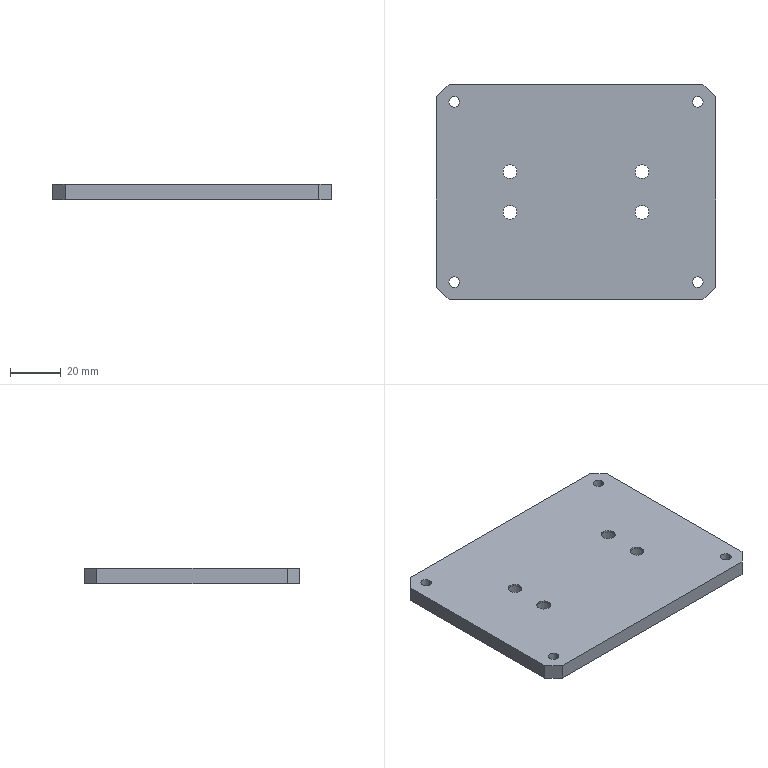Part | SolidWorks | features HoleWzd 2, Chamfer 1, Extrusion 1 | 1 solid | 38 faces | box 110 x 85 x 6 mm | volume 53736 mm3 | cylinder 24 | plane 14 | commonest cylinder face diameters 4.2 x8 5.5 x8 10 x8
STEP:
#1=CARTESIAN_POINT('',(-71.134,24.385,0.));
#2=VERTEX_POINT('',#1);
#3=CARTESIAN_POINT('',(-66.934,24.385,0.));
#4=VERTEX_POINT('',#3);
#5=CARTESIAN_POINT('',(-69.034,24.385,0.));
#6=DIRECTION('',(0.,0.,1.));
#7=DIRECTION('',(1.,0.,0.));
#8=AXIS2_PLACEMENT_3D('',#5,#6,#7);
#9=CIRCLE('',#8,2.1);
#10=EDGE_CURVE('',#2,#4,#9,.T.);
#11=ORIENTED_EDGE('',*,*,#10,.F.);
#12=CARTESIAN_POINT('',(-71.134,24.385,6.));
#13=VERTEX_POINT('',#12);
#14=CARTESIAN_POINT('',(-71.134,24.385,6.));
#15=DIRECTION('',(0.,0.,1.));
#16=VECTOR('',#15,1000.);
#17=LINE('',#14,#16);
#18=EDGE_CURVE('',#2,#13,#17,.T.);
#19=ORIENTED_EDGE('',*,*,#18,.T.);
#20=CARTESIAN_POINT('',(-66.934,24.385,6.));
#21=VERTEX_POINT('',#20);
#22=CARTESIAN_POINT('',(-69.034,24.385,6.));
#23=DIRECTION('',(0.,0.,1.));
#24=DIRECTION('',(1.,0.,0.));
#25=AXIS2_PLACEMENT_3D('',#22,#23,#24);
#26=CIRCLE('',#25,2.1);
#27=EDGE_CURVE('',#13,#21,#26,.T.);
#28=ORIENTED_EDGE('',*,*,#27,.T.);
#29=CARTESIAN_POINT('',(-66.934,24.385,6.));
#30=DIRECTION('',(0.,0.,1.));
#31=VECTOR('',#30,1000.);
#32=LINE('',#29,#31);
#33=EDGE_CURVE('',#4,#21,#32,.T.);
#34=ORIENTED_EDGE('',*,*,#33,.F.);
#35=EDGE_LOOP('',(#11,#19,#28,#34));
#36=FACE_OUTER_BOUND('',#35,.T.);
#37=CARTESIAN_POINT('',(-69.034,24.385,6.));
#38=DIRECTION('',(0.,0.,1.));
#39=DIRECTION('',(1.,0.,0.));
#40=AXIS2_PLACEMENT_3D('',#37,#38,#39);
#41=CYLINDRICAL_SURFACE('',#40,2.1);
#42=ADVANCED_FACE('',(#36),#41,.F.);
#43=CARTESIAN_POINT('',(24.866,24.385,0.));
#44=VERTEX_POINT('',#43);
#45=CARTESIAN_POINT('',(29.066,24.385,0.));
#46=VERTEX_POINT('',#45);
#47=CARTESIAN_POINT('',(26.966,24.385,0.));
#48=DIRECTION('',(0.,0.,1.));
#49=DIRECTION('',(1.,0.,0.));
#50=AXIS2_PLACEMENT_3D('',#47,#48,#49);
#51=CIRCLE('',#50,2.1);
#52=EDGE_CURVE('',#44,#46,#51,.T.);
#53=ORIENTED_EDGE('',*,*,#52,.F.);
#54=CARTESIAN_POINT('',(24.866,24.385,6.));
#55=VERTEX_POINT('',#54);
#56=CARTESIAN_POINT('',(24.866,24.385,6.));
#57=DIRECTION('',(0.,0.,1.));
#58=VECTOR('',#57,1000.);
#59=LINE('',#56,#58);
#60=EDGE_CURVE('',#44,#55,#59,.T.);
#61=ORIENTED_EDGE('',*,*,#60,.T.);
#62=CARTESIAN_POINT('',(29.066,24.385,6.));
#63=VERTEX_POINT('',#62);
#64=CARTESIAN_POINT('',(26.966,24.385,6.));
#65=DIRECTION('',(0.,0.,1.));
#66=DIRECTION('',(1.,0.,0.));
#67=AXIS2_PLACEMENT_3D('',#64,#65,#66);
#68=CIRCLE('',#67,2.1);
#69=EDGE_CURVE('',#55,#63,#68,.T.);
#70=ORIENTED_EDGE('',*,*,#69,.T.);
#71=CARTESIAN_POINT('',(29.066,24.385,6.));
#72=DIRECTION('',(0.,0.,1.));
#73=VECTOR('',#72,1000.);
#74=LINE('',#71,#73);
#75=EDGE_CURVE('',#46,#63,#74,.T.);
#76=ORIENTED_EDGE('',*,*,#75,.F.);
#77=EDGE_LOOP('',(#53,#61,#70,#76));
#78=FACE_OUTER_BOUND('',#77,.T.);
#79=CARTESIAN_POINT('',(26.966,24.385,6.));
#80=DIRECTION('',(0.,0.,1.));
#81=DIRECTION('',(1.,0.,0.));
#82=AXIS2_PLACEMENT_3D('',#79,#80,#81);
#83=CYLINDRICAL_SURFACE('',#82,2.1);
#84=ADVANCED_FACE('',(#78),#83,.F.);
#85=CARTESIAN_POINT('',(24.866,-46.615,0.));
#86=VERTEX_POINT('',#85);
#87=CARTESIAN_POINT('',(29.066,-46.615,0.));
#88=VERTEX_POINT('',#87);
#89=CARTESIAN_POINT('',(26.966,-46.615,0.));
#90=DIRECTION('',(0.,0.,1.));
#91=DIRECTION('',(1.,0.,0.));
#92=AXIS2_PLACEMENT_3D('',#89,#90,#91);
#93=CIRCLE('',#92,2.1);
#94=EDGE_CURVE('',#86,#88,#93,.T.);
#95=ORIENTED_EDGE('',*,*,#94,.F.);
#96=CARTESIAN_POINT('',(24.866,-46.615,6.));
#97=VERTEX_POINT('',#96);
#98=CARTESIAN_POINT('',(24.866,-46.615,6.));
#99=DIRECTION('',(0.,0.,1.));
#100=VECTOR('',#99,1000.);
#101=LINE('',#98,#100);
#102=EDGE_CURVE('',#86,#97,#101,.T.);
#103=ORIENTED_EDGE('',*,*,#102,.T.);
#104=CARTESIAN_POINT('',(29.066,-46.615,6.));
#105=VERTEX_POINT('',#104);
#106=CARTESIAN_POINT('',(26.966,-46.615,6.));
#107=DIRECTION('',(0.,0.,1.));
#108=DIRECTION('',(1.,0.,0.));
#109=AXIS2_PLACEMENT_3D('',#106,#107,#108);
#110=CIRCLE('',#109,2.1);
#111=EDGE_CURVE('',#97,#105,#110,.T.);
#112=ORIENTED_EDGE('',*,*,#111,.T.);
#113=CARTESIAN_POINT('',(29.066,-46.615,6.));
#114=DIRECTION('',(0.,0.,1.));
#115=VECTOR('',#114,1000.);
#116=LINE('',#113,#115);
#117=EDGE_CURVE('',#88,#105,#116,.T.);
#118=ORIENTED_EDGE('',*,*,#117,.F.);
#119=EDGE_LOOP('',(#95,#103,#112,#118));
#120=FACE_OUTER_BOUND('',#119,.T.);
#121=CARTESIAN_POINT('',(26.966,-46.615,6.));
#122=DIRECTION('',(0.,0.,1.));
#123=DIRECTION('',(1.,0.,0.));
#124=AXIS2_PLACEMENT_3D('',#121,#122,#123);
#125=CYLINDRICAL_SURFACE('',#124,2.1);
#126=ADVANCED_FACE('',(#120),#125,.F.);
#127=CARTESIAN_POINT('',(-71.134,-46.615,0.));
#128=VERTEX_POINT('',#127);
#129=CARTESIAN_POINT('',(-66.934,-46.615,0.));
#130=VERTEX_POINT('',#129);
#131=CARTESIAN_POINT('',(-69.034,-46.615,0.));
#132=DIRECTION('',(0.,0.,1.));
#133=DIRECTION('',(1.,0.,0.));
#134=AXIS2_PLACEMENT_3D('',#131,#132,#133);
#135=CIRCLE('',#134,2.1);
#136=EDGE_CURVE('',#128,#130,#135,.T.);
#137=ORIENTED_EDGE('',*,*,#136,.F.);
#138=CARTESIAN_POINT('',(-71.134,-46.615,6.));
#139=VERTEX_POINT('',#138);
#140=CARTESIAN_POINT('',(-71.134,-46.615,6.));
#141=DIRECTION('',(0.,0.,1.));
#142=VECTOR('',#141,1000.);
#143=LINE('',#140,#142);
#144=EDGE_CURVE('',#128,#139,#143,.T.);
#145=ORIENTED_EDGE('',*,*,#144,.T.);
#146=CARTESIAN_POINT('',(-66.934,-46.615,6.));
#147=VERTEX_POINT('',#146);
#148=CARTESIAN_POINT('',(-69.034,-46.615,6.));
#149=DIRECTION('',(0.,0.,1.));
#150=DIRECTION('',(1.,0.,0.));
#151=AXIS2_PLACEMENT_3D('',#148,#149,#150);
#152=CIRCLE('',#151,2.1);
#153=EDGE_CURVE('',#139,#147,#152,.T.);
#154=ORIENTED_EDGE('',*,*,#153,.T.);
#155=CARTESIAN_POINT('',(-66.934,-46.615,6.));
#156=DIRECTION('',(0.,0.,1.));
#157=VECTOR('',#156,1000.);
#158=LINE('',#155,#157);
#159=EDGE_CURVE('',#130,#147,#158,.T.);
#160=ORIENTED_EDGE('',*,*,#159,.F.);
#161=EDGE_LOOP('',(#137,#145,#154,#160));
#162=FACE_OUTER_BOUND('',#161,.T.);
#163=CARTESIAN_POINT('',(-69.034,-46.615,6.));
#164=DIRECTION('',(0.,0.,1.));
#165=DIRECTION('',(1.,0.,0.));
#166=AXIS2_PLACEMENT_3D('',#163,#164,#165);
#167=CYLINDRICAL_SURFACE('',#166,2.1);
#168=ADVANCED_FACE('',(#162),#167,.F.);
#169=CARTESIAN_POINT('',(-42.034,-19.115,5.3));
#170=VERTEX_POINT('',#169);
#171=CARTESIAN_POINT('',(-52.034,-19.115,5.3));
#172=VERTEX_POINT('',#171);
#173=CARTESIAN_POINT('',(-47.034,-19.115,5.3));
#174=DIRECTION('',(0.,0.,-1.));
#175=DIRECTION('',(-1.,0.,0.));
#176=AXIS2_PLACEMENT_3D('',#173,#174,#175);
#177=CIRCLE('',#176,5.);
#178=EDGE_CURVE('',#170,#172,#177,.T.);
#179=ORIENTED_EDGE('',*,*,#178,.F.);
#180=CARTESIAN_POINT('',(-42.034,-19.115,0.));
#181=VERTEX_POINT('',#180);
#182=CARTESIAN_POINT('',(-42.034,-19.115,0.));
#183=DIRECTION('',(0.,0.,-1.));
#184=VECTOR('',#183,1000.);
#185=LINE('',#182,#184);
#186=EDGE_CURVE('',#170,#181,#185,.T.);
#187=ORIENTED_EDGE('',*,*,#186,.T.);
#188=CARTESIAN_POINT('',(-52.034,-19.115,0.));
#189=VERTEX_POINT('',#188);
#190=CARTESIAN_POINT('',(-47.034,-19.115,0.));
#191=DIRECTION('',(0.,0.,-1.));
#192=DIRECTION('',(-1.,0.,0.));
#193=AXIS2_PLACEMENT_3D('',#190,#191,#192);
#194=CIRCLE('',#193,5.);
#195=EDGE_CURVE('',#181,#189,#194,.T.);
#196=ORIENTED_EDGE('',*,*,#195,.T.);
#197=CARTESIAN_POINT('',(-52.034,-19.115,0.));
#198=DIRECTION('',(0.,0.,-1.));
#199=VECTOR('',#198,1000.);
#200=LINE('',#197,#199);
#201=EDGE_CURVE('',#172,#189,#200,.T.);
#202=ORIENTED_EDGE('',*,*,#201,.F.);
#203=EDGE_LOOP('',(#179,#187,#196,#202));
#204=FACE_OUTER_BOUND('',#203,.T.);
#205=CARTESIAN_POINT('',(-47.034,-19.115,0.));
#206=DIRECTION('',(0.,0.,-1.));
#207=DIRECTION('',(-1.,0.,0.));
#208=AXIS2_PLACEMENT_3D('',#205,#206,#207);
#209=CYLINDRICAL_SURFACE('',#208,5.);
#210=ADVANCED_FACE('',(#204),#209,.F.);
#211=CARTESIAN_POINT('',(-44.284,-19.115,6.));
#212=VERTEX_POINT('',#211);
#213=CARTESIAN_POINT('',(-49.784,-19.115,6.));
#214=VERTEX_POINT('',#213);
#215=CARTESIAN_POINT('',(-47.034,-19.115,6.));
#216=DIRECTION('',(0.,0.,-1.));
#217=DIRECTION('',(-1.,0.,0.));
#218=AXIS2_PLACEMENT_3D('',#215,#216,#217);
#219=CIRCLE('',#218,2.75);
#220=EDGE_CURVE('',#212,#214,#219,.T.);
#221=ORIENTED_EDGE('',*,*,#220,.F.);
#222=CARTESIAN_POINT('',(-44.284,-19.115,5.3));
#223=VERTEX_POINT('',#222);
#224=CARTESIAN_POINT('',(-44.284,-19.115,0.));
#225=DIRECTION('',(0.,0.,-1.));
#226=VECTOR('',#225,1000.);
#227=LINE('',#224,#226);
#228=EDGE_CURVE('',#212,#223,#227,.T.);
#229=ORIENTED_EDGE('',*,*,#228,.T.);
#230=CARTESIAN_POINT('',(-49.784,-19.115,5.3));
#231=VERTEX_POINT('',#230);
#232=CARTESIAN_POINT('',(-47.034,-19.115,5.3));
#233=DIRECTION('',(0.,0.,-1.));
#234=DIRECTION('',(-1.,0.,0.));
#235=AXIS2_PLACEMENT_3D('',#232,#233,#234);
#236=CIRCLE('',#235,2.75);
#237=EDGE_CURVE('',#223,#231,#236,.T.);
#238=ORIENTED_EDGE('',*,*,#237,.T.);
#239=CARTESIAN_POINT('',(-49.784,-19.115,0.));
#240=DIRECTION('',(0.,0.,-1.));
#241=VECTOR('',#240,1000.);
#242=LINE('',#239,#241);
#243=EDGE_CURVE('',#214,#231,#242,.T.);
#244=ORIENTED_EDGE('',*,*,#243,.F.);
#245=EDGE_LOOP('',(#221,#229,#238,#244));
#246=FACE_OUTER_BOUND('',#245,.T.);
#247=CARTESIAN_POINT('',(-47.034,-19.115,0.));
#248=DIRECTION('',(0.,0.,-1.));
#249=DIRECTION('',(-1.,0.,0.));
#250=AXIS2_PLACEMENT_3D('',#247,#248,#249);
#251=CYLINDRICAL_SURFACE('',#250,2.75);
#252=ADVANCED_FACE('',(#246),#251,.F.);
#253=CARTESIAN_POINT('',(9.966,-19.115,5.3));
#254=VERTEX_POINT('',#253);
#255=CARTESIAN_POINT('',(-0.03364,-19.115,5.3));
#256=VERTEX_POINT('',#255);
#257=CARTESIAN_POINT('',(4.966,-19.115,5.3));
#258=DIRECTION('',(0.,0.,-1.));
#259=DIRECTION('',(-1.,0.,0.));
#260=AXIS2_PLACEMENT_3D('',#257,#258,#259);
#261=CIRCLE('',#260,5.);
#262=EDGE_CURVE('',#254,#256,#261,.T.);
#263=ORIENTED_EDGE('',*,*,#262,.F.);
#264=CARTESIAN_POINT('',(9.966,-19.115,0.));
#265=VERTEX_POINT('',#264);
#266=CARTESIAN_POINT('',(9.966,-19.115,0.));
#267=DIRECTION('',(0.,0.,-1.));
#268=VECTOR('',#267,1000.);
#269=LINE('',#266,#268);
#270=EDGE_CURVE('',#254,#265,#269,.T.);
#271=ORIENTED_EDGE('',*,*,#270,.T.);
#272=CARTESIAN_POINT('',(-0.03364,-19.115,0.));
#273=VERTEX_POINT('',#272);
#274=CARTESIAN_POINT('',(4.966,-19.115,0.));
#275=DIRECTION('',(0.,0.,-1.));
#276=DIRECTION('',(-1.,0.,0.));
#277=AXIS2_PLACEMENT_3D('',#274,#275,#276);
#278=CIRCLE('',#277,5.);
#279=EDGE_CURVE('',#265,#273,#278,.T.);
#280=ORIENTED_EDGE('',*,*,#279,.T.);
#281=CARTESIAN_POINT('',(-0.03364,-19.115,0.));
#282=DIRECTION('',(0.,0.,-1.));
#283=VECTOR('',#282,1000.);
#284=LINE('',#281,#283);
#285=EDGE_CURVE('',#256,#273,#284,.T.);
#286=ORIENTED_EDGE('',*,*,#285,.F.);
#287=EDGE_LOOP('',(#263,#271,#280,#286));
#288=FACE_OUTER_BOUND('',#287,.T.);
#289=CARTESIAN_POINT('',(4.966,-19.115,0.));
#290=DIRECTION('',(0.,0.,-1.));
#291=DIRECTION('',(-1.,0.,0.));
#292=AXIS2_PLACEMENT_3D('',#289,#290,#291);
#293=CYLINDRICAL_SURFACE('',#292,5.);
#294=ADVANCED_FACE('',(#288),#293,.F.);
#295=CARTESIAN_POINT('',(7.716,-19.115,6.));
#296=VERTEX_POINT('',#295);
#297=CARTESIAN_POINT('',(2.216,-19.115,6.));
#298=VERTEX_POINT('',#297);
#299=CARTESIAN_POINT('',(4.966,-19.115,6.));
#300=DIRECTION('',(0.,0.,-1.));
#301=DIRECTION('',(-1.,0.,0.));
#302=AXIS2_PLACEMENT_3D('',#299,#300,#301);
#303=CIRCLE('',#302,2.75);
#304=EDGE_CURVE('',#296,#298,#303,.T.);
#305=ORIENTED_EDGE('',*,*,#304,.F.);
#306=CARTESIAN_POINT('',(7.716,-19.115,5.3));
#307=VERTEX_POINT('',#306);
#308=CARTESIAN_POINT('',(7.716,-19.115,0.));
#309=DIRECTION('',(0.,0.,-1.));
#310=VECTOR('',#309,1000.);
#311=LINE('',#308,#310);
#312=EDGE_CURVE('',#296,#307,#311,.T.);
#313=ORIENTED_EDGE('',*,*,#312,.T.);
#314=CARTESIAN_POINT('',(2.216,-19.115,5.3));
#315=VERTEX_POINT('',#314);
#316=CARTESIAN_POINT('',(4.966,-19.115,5.3));
#317=DIRECTION('',(0.,0.,-1.));
#318=DIRECTION('',(-1.,0.,0.));
#319=AXIS2_PLACEMENT_3D('',#316,#317,#318);
#320=CIRCLE('',#319,2.75);
#321=EDGE_CURVE('',#307,#315,#320,.T.);
#322=ORIENTED_EDGE('',*,*,#321,.T.);
#323=CARTESIAN_POINT('',(2.216,-19.115,0.));
#324=DIRECTION('',(0.,0.,-1.));
#325=VECTOR('',#324,1000.);
#326=LINE('',#323,#325);
#327=EDGE_CURVE('',#298,#315,#326,.T.);
#328=ORIENTED_EDGE('',*,*,#327,.F.);
#329=EDGE_LOOP('',(#305,#313,#322,#328));
#330=FACE_OUTER_BOUND('',#329,.T.);
#331=CARTESIAN_POINT('',(4.966,-19.115,0.));
#332=DIRECTION('',(0.,0.,-1.));
#333=DIRECTION('',(-1.,0.,0.));
#334=AXIS2_PLACEMENT_3D('',#331,#332,#333);
#335=CYLINDRICAL_SURFACE('',#334,2.75);
#336=ADVANCED_FACE('',(#330),#335,.F.);
#337=CARTESIAN_POINT('',(9.966,-3.115,5.3));
#338=VERTEX_POINT('',#337);
#339=CARTESIAN_POINT('',(-0.03364,-3.115,5.3));
#340=VERTEX_POINT('',#339);
#341=CARTESIAN_POINT('',(4.966,-3.115,5.3));
#342=DIRECTION('',(0.,0.,-1.));
#343=DIRECTION('',(-1.,0.,0.));
#344=AXIS2_PLACEMENT_3D('',#341,#342,#343);
#345=CIRCLE('',#344,5.);
#346=EDGE_CURVE('',#338,#340,#345,.T.);
#347=ORIENTED_EDGE('',*,*,#346,.F.);
#348=CARTESIAN_POINT('',(9.966,-3.115,0.));
#349=VERTEX_POINT('',#348);
#350=CARTESIAN_POINT('',(9.966,-3.115,0.));
#351=DIRECTION('',(0.,0.,-1.));
#352=VECTOR('',#351,1000.);
#353=LINE('',#350,#352);
#354=EDGE_CURVE('',#338,#349,#353,.T.);
#355=ORIENTED_EDGE('',*,*,#354,.T.);
#356=CARTESIAN_POINT('',(-0.03364,-3.115,0.));
#357=VERTEX_POINT('',#356);
#358=CARTESIAN_POINT('',(4.966,-3.115,0.));
#359=DIRECTION('',(0.,0.,-1.));
#360=DIRECTION('',(-1.,0.,0.));
#361=AXIS2_PLACEMENT_3D('',#358,#359,#360);
#362=CIRCLE('',#361,5.);
#363=EDGE_CURVE('',#349,#357,#362,.T.);
#364=ORIENTED_EDGE('',*,*,#363,.T.);
#365=CARTESIAN_POINT('',(-0.03364,-3.115,0.));
#366=DIRECTION('',(0.,0.,-1.));
#367=VECTOR('',#366,1000.);
#368=LINE('',#365,#367);
#369=EDGE_CURVE('',#340,#357,#368,.T.);
#370=ORIENTED_EDGE('',*,*,#369,.F.);
#371=EDGE_LOOP('',(#347,#355,#364,#370));
#372=FACE_OUTER_BOUND('',#371,.T.);
#373=CARTESIAN_POINT('',(4.966,-3.115,0.));
#374=DIRECTION('',(0.,0.,-1.));
#375=DIRECTION('',(-1.,0.,0.));
#376=AXIS2_PLACEMENT_3D('',#373,#374,#375);
#377=CYLINDRICAL_SURFACE('',#376,5.);
#378=ADVANCED_FACE('',(#372),#377,.F.);
#379=CARTESIAN_POINT('',(7.716,-3.115,6.));
#380=VERTEX_POINT('',#379);
#381=CARTESIAN_POINT('',(2.216,-3.115,6.));
#382=VERTEX_POINT('',#381);
#383=CARTESIAN_POINT('',(4.966,-3.115,6.));
#384=DIRECTION('',(0.,0.,-1.));
#385=DIRECTION('',(-1.,0.,0.));
#386=AXIS2_PLACEMENT_3D('',#383,#384,#385);
#387=CIRCLE('',#386,2.75);
#388=EDGE_CURVE('',#380,#382,#387,.T.);
#389=ORIENTED_EDGE('',*,*,#388,.F.);
#390=CARTESIAN_POINT('',(7.716,-3.115,5.3));
#391=VERTEX_POINT('',#390);
#392=CARTESIAN_POINT('',(7.716,-3.115,0.));
#393=DIRECTION('',(0.,0.,-1.));
#394=VECTOR('',#393,1000.);
#395=LINE('',#392,#394);
#396=EDGE_CURVE('',#380,#391,#395,.T.);
#397=ORIENTED_EDGE('',*,*,#396,.T.);
#398=CARTESIAN_POINT('',(2.216,-3.115,5.3));
#399=VERTEX_POINT('',#398);
#400=CARTESIAN_POINT('',(4.966,-3.115,5.3));
#401=DIRECTION('',(0.,0.,-1.));
#402=DIRECTION('',(-1.,0.,0.));
#403=AXIS2_PLACEMENT_3D('',#400,#401,#402);
#404=CIRCLE('',#403,2.75);
#405=EDGE_CURVE('',#391,#399,#404,.T.);
#406=ORIENTED_EDGE('',*,*,#405,.T.);
#407=CARTESIAN_POINT('',(2.216,-3.115,0.));
#408=DIRECTION('',(0.,0.,-1.));
#409=VECTOR('',#408,1000.);
#410=LINE('',#407,#409);
#411=EDGE_CURVE('',#382,#399,#410,.T.);
#412=ORIENTED_EDGE('',*,*,#411,.F.);
#413=EDGE_LOOP('',(#389,#397,#406,#412));
#414=FACE_OUTER_BOUND('',#413,.T.);
#415=CARTESIAN_POINT('',(4.966,-3.115,0.));
#416=DIRECTION('',(0.,0.,-1.));
#417=DIRECTION('',(-1.,0.,0.));
#418=AXIS2_PLACEMENT_3D('',#415,#416,#417);
#419=CYLINDRICAL_SURFACE('',#418,2.75);
#420=ADVANCED_FACE('',(#414),#419,.F.);
#421=CARTESIAN_POINT('',(-42.034,-3.115,5.3));
#422=VERTEX_POINT('',#421);
#423=CARTESIAN_POINT('',(-52.034,-3.115,5.3));
#424=VERTEX_POINT('',#423);
#425=CARTESIAN_POINT('',(-47.034,-3.115,5.3));
#426=DIRECTION('',(0.,0.,-1.));
#427=DIRECTION('',(-1.,0.,0.));
#428=AXIS2_PLACEMENT_3D('',#425,#426,#427);
#429=CIRCLE('',#428,5.);
#430=EDGE_CURVE('',#422,#424,#429,.T.);
#431=ORIENTED_EDGE('',*,*,#430,.F.);
#432=CARTESIAN_POINT('',(-42.034,-3.115,0.));
#433=VERTEX_POINT('',#432);
#434=CARTESIAN_POINT('',(-42.034,-3.115,0.));
#435=DIRECTION('',(0.,0.,-1.));
#436=VECTOR('',#435,1000.);
#437=LINE('',#434,#436);
#438=EDGE_CURVE('',#422,#433,#437,.T.);
#439=ORIENTED_EDGE('',*,*,#438,.T.);
#440=CARTESIAN_POINT('',(-52.034,-3.115,0.));
#441=VERTEX_POINT('',#440);
#442=CARTESIAN_POINT('',(-47.034,-3.115,0.));
#443=DIRECTION('',(0.,0.,-1.));
#444=DIRECTION('',(-1.,0.,0.));
#445=AXIS2_PLACEMENT_3D('',#442,#443,#444);
#446=CIRCLE('',#445,5.);
#447=EDGE_CURVE('',#433,#441,#446,.T.);
#448=ORIENTED_EDGE('',*,*,#447,.T.);
#449=CARTESIAN_POINT('',(-52.034,-3.115,0.));
#450=DIRECTION('',(0.,0.,-1.));
#451=VECTOR('',#450,1000.);
#452=LINE('',#449,#451);
#453=EDGE_CURVE('',#424,#441,#452,.T.);
#454=ORIENTED_EDGE('',*,*,#453,.F.);
#455=EDGE_LOOP('',(#431,#439,#448,#454));
#456=FACE_OUTER_BOUND('',#455,.T.);
#457=CARTESIAN_POINT('',(-47.034,-3.115,0.));
#458=DIRECTION('',(0.,0.,-1.));
#459=DIRECTION('',(-1.,0.,0.));
#460=AXIS2_PLACEMENT_3D('',#457,#458,#459);
#461=CYLINDRICAL_SURFACE('',#460,5.);
#462=ADVANCED_FACE('',(#456),#461,.F.);
#463=CARTESIAN_POINT('',(-44.284,-3.115,6.));
#464=VERTEX_POINT('',#463);
#465=CARTESIAN_POINT('',(-49.784,-3.115,6.));
#466=VERTEX_POINT('',#465);
#467=CARTESIAN_POINT('',(-47.034,-3.115,6.));
#468=DIRECTION('',(0.,0.,-1.));
#469=DIRECTION('',(-1.,0.,0.));
#470=AXIS2_PLACEMENT_3D('',#467,#468,#469);
#471=CIRCLE('',#470,2.75);
#472=EDGE_CURVE('',#464,#466,#471,.T.);
#473=ORIENTED_EDGE('',*,*,#472,.F.);
#474=CARTESIAN_POINT('',(-44.284,-3.115,5.3));
#475=VERTEX_POINT('',#474);
#476=CARTESIAN_POINT('',(-44.284,-3.115,0.));
#477=DIRECTION('',(0.,0.,-1.));
#478=VECTOR('',#477,1000.);
#479=LINE('',#476,#478);
#480=EDGE_CURVE('',#464,#475,#479,.T.);
#481=ORIENTED_EDGE('',*,*,#480,.T.);
#482=CARTESIAN_POINT('',(-49.784,-3.115,5.3));
#483=VERTEX_POINT('',#482);
#484=CARTESIAN_POINT('',(-47.034,-3.115,5.3));
#485=DIRECTION('',(0.,0.,-1.));
#486=DIRECTION('',(-1.,0.,0.));
#487=AXIS2_PLACEMENT_3D('',#484,#485,#486);
#488=CIRCLE('',#487,2.75);
#489=EDGE_CURVE('',#475,#483,#488,.T.);
#490=ORIENTED_EDGE('',*,*,#489,.T.);
#491=CARTESIAN_POINT('',(-49.784,-3.115,0.));
#492=DIRECTION('',(0.,0.,-1.));
#493=VECTOR('',#492,1000.);
#494=LINE('',#491,#493);
#495=EDGE_CURVE('',#466,#483,#494,.T.);
#496=ORIENTED_EDGE('',*,*,#495,.F.);
#497=EDGE_LOOP('',(#473,#481,#490,#496));
#498=FACE_OUTER_BOUND('',#497,.T.);
#499=CARTESIAN_POINT('',(-47.034,-3.115,0.));
#500=DIRECTION('',(0.,0.,-1.));
#501=DIRECTION('',(-1.,0.,0.));
#502=AXIS2_PLACEMENT_3D('',#499,#500,#501);
#503=CYLINDRICAL_SURFACE('',#502,2.75);
#504=ADVANCED_FACE('',(#498),#503,.F.);
#505=CARTESIAN_POINT('',(-76.034,26.385,6.));
#506=VERTEX_POINT('',#505);
#507=CARTESIAN_POINT('',(-76.034,-48.615,6.));
#508=VERTEX_POINT('',#507);
#509=CARTESIAN_POINT('',(-76.034,31.385,6.));
#510=DIRECTION('',(0.,-1.,0.));
#511=VECTOR('',#510,1000.);
#512=LINE('',#509,#511);
#513=EDGE_CURVE('',#506,#508,#512,.T.);
#514=ORIENTED_EDGE('',*,*,#513,.F.);
#515=CARTESIAN_POINT('',(-76.034,26.385,0.));
#516=VERTEX_POINT('',#515);
#517=CARTESIAN_POINT('',(-76.034,26.385,6.));
#518=DIRECTION('',(0.,0.,-1.));
#519=VECTOR('',#518,1000.);
#520=LINE('',#517,#519);
#521=EDGE_CURVE('',#506,#516,#520,.T.);
#522=ORIENTED_EDGE('',*,*,#521,.T.);
#523=CARTESIAN_POINT('',(-76.034,-48.615,0.));
#524=VERTEX_POINT('',#523);
#525=CARTESIAN_POINT('',(-76.034,31.385,0.));
#526=DIRECTION('',(0.,-1.,0.));
#527=VECTOR('',#526,1000.);
#528=LINE('',#525,#527);
#529=EDGE_CURVE('',#516,#524,#528,.T.);
#530=ORIENTED_EDGE('',*,*,#529,.T.);
#531=CARTESIAN_POINT('',(-76.034,-48.615,6.));
#532=DIRECTION('',(0.,0.,1.));
#533=VECTOR('',#532,1000.);
#534=LINE('',#531,#533);
#535=EDGE_CURVE('',#524,#508,#534,.T.);
#536=ORIENTED_EDGE('',*,*,#535,.T.);
#537=EDGE_LOOP('',(#514,#522,#530,#536));
#538=FACE_OUTER_BOUND('',#537,.T.);
#539=CARTESIAN_POINT('',(-76.034,31.385,6.));
#540=DIRECTION('',(1.,0.,0.));
#541=DIRECTION('',(0.,1.,0.));
#542=AXIS2_PLACEMENT_3D('',#539,#540,#541);
#543=PLANE('',#542);
#544=ADVANCED_FACE('',(#538),#543,.F.);
#545=CARTESIAN_POINT('',(-71.034,-53.615,6.));
#546=VERTEX_POINT('',#545);
#547=CARTESIAN_POINT('',(28.966,-53.615,6.));
#548=VERTEX_POINT('',#547);
#549=CARTESIAN_POINT('',(-76.034,-53.615,6.));
#550=DIRECTION('',(1.,0.,0.));
#551=VECTOR('',#550,1000.);
#552=LINE('',#549,#551);
#553=EDGE_CURVE('',#546,#548,#552,.T.);
#554=ORIENTED_EDGE('',*,*,#553,.F.);
#555=CARTESIAN_POINT('',(-71.034,-53.615,0.));
#556=VERTEX_POINT('',#555);
#557=CARTESIAN_POINT('',(-71.034,-53.615,6.));
#558=DIRECTION('',(0.,0.,-1.));
#559=VECTOR('',#558,1000.);
#560=LINE('',#557,#559);
#561=EDGE_CURVE('',#546,#556,#560,.T.);
#562=ORIENTED_EDGE('',*,*,#561,.T.);
#563=CARTESIAN_POINT('',(28.966,-53.615,0.));
#564=VERTEX_POINT('',#563);
#565=CARTESIAN_POINT('',(-76.034,-53.615,0.));
#566=DIRECTION('',(1.,0.,0.));
#567=VECTOR('',#566,1000.);
#568=LINE('',#565,#567);
#569=EDGE_CURVE('',#556,#564,#568,.T.);
#570=ORIENTED_EDGE('',*,*,#569,.T.);
#571=CARTESIAN_POINT('',(28.966,-53.615,6.));
#572=DIRECTION('',(0.,0.,1.));
#573=VECTOR('',#572,1000.);
#574=LINE('',#571,#573);
#575=EDGE_CURVE('',#564,#548,#574,.T.);
#576=ORIENTED_EDGE('',*,*,#575,.T.);
#577=EDGE_LOOP('',(#554,#562,#570,#576));
#578=FACE_OUTER_BOUND('',#577,.T.);
#579=CARTESIAN_POINT('',(-76.034,-53.615,6.));
#580=DIRECTION('',(0.,1.,0.));
#581=DIRECTION('',(0.,0.,1.));
#582=AXIS2_PLACEMENT_3D('',#579,#580,#581);
#583=PLANE('',#582);
#584=ADVANCED_FACE('',(#578),#583,.F.);
#585=CARTESIAN_POINT('',(33.966,-48.615,6.));
#586=VERTEX_POINT('',#585);
#587=CARTESIAN_POINT('',(33.966,26.385,6.));
#588=VERTEX_POINT('',#587);
#589=CARTESIAN_POINT('',(33.966,31.385,6.));
#590=DIRECTION('',(0.,1.,0.));
#591=VECTOR('',#590,1000.);
#592=LINE('',#589,#591);
#593=EDGE_CURVE('',#586,#588,#592,.T.);
#594=ORIENTED_EDGE('',*,*,#593,.F.);
#595=CARTESIAN_POINT('',(33.966,-48.615,0.));
#596=VERTEX_POINT('',#595);
#597=CARTESIAN_POINT('',(33.966,-48.615,6.));
#598=DIRECTION('',(0.,0.,-1.));
#599=VECTOR('',#598,1000.);
#600=LINE('',#597,#599);
#601=EDGE_CURVE('',#586,#596,#600,.T.);
#602=ORIENTED_EDGE('',*,*,#601,.T.);
#603=CARTESIAN_POINT('',(33.966,26.385,0.));
#604=VERTEX_POINT('',#603);
#605=CARTESIAN_POINT('',(33.966,31.385,0.));
#606=DIRECTION('',(0.,1.,0.));
#607=VECTOR('',#606,1000.);
#608=LINE('',#605,#607);
#609=EDGE_CURVE('',#596,#604,#608,.T.);
#610=ORIENTED_EDGE('',*,*,#609,.T.);
#611=CARTESIAN_POINT('',(33.966,26.385,6.));
#612=DIRECTION('',(0.,0.,1.));
#613=VECTOR('',#612,1000.);
#614=LINE('',#611,#613);
#615=EDGE_CURVE('',#604,#588,#614,.T.);
#616=ORIENTED_EDGE('',*,*,#615,.T.);
#617=EDGE_LOOP('',(#594,#602,#610,#616));
#618=FACE_OUTER_BOUND('',#617,.T.);
#619=CARTESIAN_POINT('',(33.966,31.385,6.));
#620=DIRECTION('',(-1.,0.,0.));
#621=DIRECTION('',(0.,-1.,0.));
#622=AXIS2_PLACEMENT_3D('',#619,#620,#621);
#623=PLANE('',#622);
#624=ADVANCED_FACE('',(#618),#623,.F.);
#625=CARTESIAN_POINT('',(28.966,31.385,0.));
#626=VERTEX_POINT('',#625);
#627=CARTESIAN_POINT('',(-71.034,31.385,0.));
#628=VERTEX_POINT('',#627);
#629=CARTESIAN_POINT('',(-76.034,31.385,0.));
#630=DIRECTION('',(-1.,0.,0.));
#631=VECTOR('',#630,1000.);
#632=LINE('',#629,#631);
#633=EDGE_CURVE('',#626,#628,#632,.T.);
#634=ORIENTED_EDGE('',*,*,#633,.T.);
#635=CARTESIAN_POINT('',(-71.034,31.385,6.));
#636=VERTEX_POINT('',#635);
#637=CARTESIAN_POINT('',(-71.034,31.385,6.));
#638=DIRECTION('',(0.,0.,1.));
#639=VECTOR('',#638,1000.);
#640=LINE('',#637,#639);
#641=EDGE_CURVE('',#628,#636,#640,.T.);
#642=ORIENTED_EDGE('',*,*,#641,.T.);
#643=CARTESIAN_POINT('',(28.966,31.385,6.));
#644=VERTEX_POINT('',#643);
#645=CARTESIAN_POINT('',(-76.034,31.385,6.));
#646=DIRECTION('',(-1.,0.,0.));
#647=VECTOR('',#646,1000.);
#648=LINE('',#645,#647);
#649=EDGE_CURVE('',#644,#636,#648,.T.);
#650=ORIENTED_EDGE('',*,*,#649,.F.);
#651=CARTESIAN_POINT('',(28.966,31.385,6.));
#652=DIRECTION('',(0.,0.,-1.));
#653=VECTOR('',#652,1000.);
#654=LINE('',#651,#653);
#655=EDGE_CURVE('',#644,#626,#654,.T.);
#656=ORIENTED_EDGE('',*,*,#655,.T.);
#657=EDGE_LOOP('',(#634,#642,#650,#656));
#658=FACE_OUTER_BOUND('',#657,.T.);
#659=CARTESIAN_POINT('',(-76.034,31.385,6.));
#660=DIRECTION('',(0.,-1.,0.));
#661=DIRECTION('',(0.,0.,-1.));
#662=AXIS2_PLACEMENT_3D('',#659,#660,#661);
#663=PLANE('',#662);
#664=ADVANCED_FACE('',(#658),#663,.F.);
#665=CARTESIAN_POINT('',(-69.034,24.385,6.));
#666=DIRECTION('',(0.,0.,1.));
#667=DIRECTION('',(1.,0.,0.));
#668=AXIS2_PLACEMENT_3D('',#665,#666,#667);
#669=CIRCLE('',#668,2.1);
#670=EDGE_CURVE('',#21,#13,#669,.T.);
#671=ORIENTED_EDGE('',*,*,#670,.F.);
#672=ORIENTED_EDGE('',*,*,#27,.F.);
#673=EDGE_LOOP('',(#671,#672));
#674=FACE_BOUND('',#673,.T.);
#675=CARTESIAN_POINT('',(26.966,24.385,6.));
#676=DIRECTION('',(0.,0.,1.));
#677=DIRECTION('',(1.,0.,0.));
#678=AXIS2_PLACEMENT_3D('',#675,#676,#677);
#679=CIRCLE('',#678,2.1);
#680=EDGE_CURVE('',#63,#55,#679,.T.);
#681=ORIENTED_EDGE('',*,*,#680,.F.);
#682=ORIENTED_EDGE('',*,*,#69,.F.);
#683=EDGE_LOOP('',(#681,#682));
#684=FACE_BOUND('',#683,.T.);
#685=CARTESIAN_POINT('',(26.966,-46.615,6.));
#686=DIRECTION('',(0.,0.,1.));
#687=DIRECTION('',(1.,0.,0.));
#688=AXIS2_PLACEMENT_3D('',#685,#686,#687);
#689=CIRCLE('',#688,2.1);
#690=EDGE_CURVE('',#105,#97,#689,.T.);
#691=ORIENTED_EDGE('',*,*,#690,.F.);
#692=ORIENTED_EDGE('',*,*,#111,.F.);
#693=EDGE_LOOP('',(#691,#692));
#694=FACE_BOUND('',#693,.T.);
#695=CARTESIAN_POINT('',(-69.034,-46.615,6.));
#696=DIRECTION('',(0.,0.,1.));
#697=DIRECTION('',(1.,0.,0.));
#698=AXIS2_PLACEMENT_3D('',#695,#696,#697);
#699=CIRCLE('',#698,2.1);
#700=EDGE_CURVE('',#147,#139,#699,.T.);
#701=ORIENTED_EDGE('',*,*,#700,.F.);
#702=ORIENTED_EDGE('',*,*,#153,.F.);
#703=EDGE_LOOP('',(#701,#702));
#704=FACE_BOUND('',#703,.T.);
#705=CARTESIAN_POINT('',(-47.034,-19.115,6.));
#706=DIRECTION('',(0.,0.,-1.));
#707=DIRECTION('',(-1.,0.,0.));
#708=AXIS2_PLACEMENT_3D('',#705,#706,#707);
#709=CIRCLE('',#708,2.75);
#710=EDGE_CURVE('',#214,#212,#709,.T.);
#711=ORIENTED_EDGE('',*,*,#710,.T.);
#712=ORIENTED_EDGE('',*,*,#220,.T.);
#713=EDGE_LOOP('',(#711,#712));
#714=FACE_BOUND('',#713,.T.);
#715=CARTESIAN_POINT('',(4.966,-19.115,6.));
#716=DIRECTION('',(0.,0.,-1.));
#717=DIRECTION('',(-1.,0.,0.));
#718=AXIS2_PLACEMENT_3D('',#715,#716,#717);
#719=CIRCLE('',#718,2.75);
#720=EDGE_CURVE('',#298,#296,#719,.T.);
#721=ORIENTED_EDGE('',*,*,#720,.T.);
#722=ORIENTED_EDGE('',*,*,#304,.T.);
#723=EDGE_LOOP('',(#721,#722));
#724=FACE_BOUND('',#723,.T.);
#725=CARTESIAN_POINT('',(4.966,-3.115,6.));
#726=DIRECTION('',(0.,0.,-1.));
#727=DIRECTION('',(-1.,0.,0.));
#728=AXIS2_PLACEMENT_3D('',#725,#726,#727);
#729=CIRCLE('',#728,2.75);
#730=EDGE_CURVE('',#382,#380,#729,.T.);
#731=ORIENTED_EDGE('',*,*,#730,.T.);
#732=ORIENTED_EDGE('',*,*,#388,.T.);
#733=EDGE_LOOP('',(#731,#732));
#734=FACE_BOUND('',#733,.T.);
#735=CARTESIAN_POINT('',(-47.034,-3.115,6.));
#736=DIRECTION('',(0.,0.,-1.));
#737=DIRECTION('',(-1.,0.,0.));
#738=AXIS2_PLACEMENT_3D('',#735,#736,#737);
#739=CIRCLE('',#738,2.75);
#740=EDGE_CURVE('',#466,#464,#739,.T.);
#741=ORIENTED_EDGE('',*,*,#740,.T.);
#742=ORIENTED_EDGE('',*,*,#472,.T.);
#743=EDGE_LOOP('',(#741,#742));
#744=FACE_BOUND('',#743,.T.);
#745=ORIENTED_EDGE('',*,*,#649,.T.);
#746=CARTESIAN_POINT('',(-51.209,51.209,6.));
#747=DIRECTION('',(-0.7071,-0.7071,0.));
#748=VECTOR('',#747,1000.);
#749=LINE('',#746,#748);
#750=EDGE_CURVE('',#636,#506,#749,.T.);
#751=ORIENTED_EDGE('',*,*,#750,.T.);
#752=ORIENTED_EDGE('',*,*,#513,.T.);
#753=CARTESIAN_POINT('',(-62.324,-62.324,6.));
#754=DIRECTION('',(0.7071,-0.7071,0.));
#755=VECTOR('',#754,1000.);
#756=LINE('',#753,#755);
#757=EDGE_CURVE('',#508,#546,#756,.T.);
#758=ORIENTED_EDGE('',*,*,#757,.T.);
#759=ORIENTED_EDGE('',*,*,#553,.T.);
#760=CARTESIAN_POINT('',(41.291,-41.291,6.));
#761=DIRECTION('',(0.7071,0.7071,0.));
#762=VECTOR('',#761,1000.);
#763=LINE('',#760,#762);
#764=EDGE_CURVE('',#548,#586,#763,.T.);
#765=ORIENTED_EDGE('',*,*,#764,.T.);
#766=ORIENTED_EDGE('',*,*,#593,.T.);
#767=CARTESIAN_POINT('',(30.176,30.176,6.));
#768=DIRECTION('',(-0.7071,0.7071,0.));
#769=VECTOR('',#768,1000.);
#770=LINE('',#767,#769);
#771=EDGE_CURVE('',#588,#644,#770,.T.);
#772=ORIENTED_EDGE('',*,*,#771,.T.);
#773=EDGE_LOOP('',(#745,#751,#752,#758,#759,#765,#766,#772));
#774=FACE_OUTER_BOUND('',#773,.T.);
#775=CARTESIAN_POINT('',(0.,0.,6.));
#776=DIRECTION('',(0.,0.,1.));
#777=DIRECTION('',(1.,0.,0.));
#778=AXIS2_PLACEMENT_3D('',#775,#776,#777);
#779=PLANE('',#778);
#780=ADVANCED_FACE('',(#674,#684,#694,#704,#714,#724,#734,#744,#774),#779,.T.);
#781=CARTESIAN_POINT('',(-69.034,24.385,0.));
#782=DIRECTION('',(0.,0.,1.));
#783=DIRECTION('',(1.,0.,0.));
#784=AXIS2_PLACEMENT_3D('',#781,#782,#783);
#785=CIRCLE('',#784,2.1);
#786=EDGE_CURVE('',#4,#2,#785,.T.);
#787=ORIENTED_EDGE('',*,*,#786,.T.);
#788=ORIENTED_EDGE('',*,*,#10,.T.);
#789=EDGE_LOOP('',(#787,#788));
#790=FACE_BOUND('',#789,.T.);
#791=CARTESIAN_POINT('',(26.966,24.385,0.));
#792=DIRECTION('',(0.,0.,1.));
#793=DIRECTION('',(1.,0.,0.));
#794=AXIS2_PLACEMENT_3D('',#791,#792,#793);
#795=CIRCLE('',#794,2.1);
#796=EDGE_CURVE('',#46,#44,#795,.T.);
#797=ORIENTED_EDGE('',*,*,#796,.T.);
#798=ORIENTED_EDGE('',*,*,#52,.T.);
#799=EDGE_LOOP('',(#797,#798));
#800=FACE_BOUND('',#799,.T.);
#801=CARTESIAN_POINT('',(26.966,-46.615,0.));
#802=DIRECTION('',(0.,0.,1.));
#803=DIRECTION('',(1.,0.,0.));
#804=AXIS2_PLACEMENT_3D('',#801,#802,#803);
#805=CIRCLE('',#804,2.1);
#806=EDGE_CURVE('',#88,#86,#805,.T.);
#807=ORIENTED_EDGE('',*,*,#806,.T.);
#808=ORIENTED_EDGE('',*,*,#94,.T.);
#809=EDGE_LOOP('',(#807,#808));
#810=FACE_BOUND('',#809,.T.);
#811=CARTESIAN_POINT('',(-69.034,-46.615,0.));
#812=DIRECTION('',(0.,0.,1.));
#813=DIRECTION('',(1.,0.,0.));
#814=AXIS2_PLACEMENT_3D('',#811,#812,#813);
#815=CIRCLE('',#814,2.1);
#816=EDGE_CURVE('',#130,#128,#815,.T.);
#817=ORIENTED_EDGE('',*,*,#816,.T.);
#818=ORIENTED_EDGE('',*,*,#136,.T.);
#819=EDGE_LOOP('',(#817,#818));
#820=FACE_BOUND('',#819,.T.);
#821=CARTESIAN_POINT('',(-47.034,-19.115,0.));
#822=DIRECTION('',(0.,0.,-1.));
#823=DIRECTION('',(-1.,0.,0.));
#824=AXIS2_PLACEMENT_3D('',#821,#822,#823);
#825=CIRCLE('',#824,5.);
#826=EDGE_CURVE('',#189,#181,#825,.T.);
#827=ORIENTED_EDGE('',*,*,#826,.F.);
#828=ORIENTED_EDGE('',*,*,#195,.F.);
#829=EDGE_LOOP('',(#827,#828));
#830=FACE_BOUND('',#829,.T.);
#831=CARTESIAN_POINT('',(4.966,-19.115,0.));
#832=DIRECTION('',(0.,0.,-1.));
#833=DIRECTION('',(-1.,0.,0.));
#834=AXIS2_PLACEMENT_3D('',#831,#832,#833);
#835=CIRCLE('',#834,5.);
#836=EDGE_CURVE('',#273,#265,#835,.T.);
#837=ORIENTED_EDGE('',*,*,#836,.F.);
#838=ORIENTED_EDGE('',*,*,#279,.F.);
#839=EDGE_LOOP('',(#837,#838));
#840=FACE_BOUND('',#839,.T.);
#841=CARTESIAN_POINT('',(4.966,-3.115,0.));
#842=DIRECTION('',(0.,0.,-1.));
#843=DIRECTION('',(-1.,0.,0.));
#844=AXIS2_PLACEMENT_3D('',#841,#842,#843);
#845=CIRCLE('',#844,5.);
#846=EDGE_CURVE('',#357,#349,#845,.T.);
#847=ORIENTED_EDGE('',*,*,#846,.F.);
#848=ORIENTED_EDGE('',*,*,#363,.F.);
#849=EDGE_LOOP('',(#847,#848));
#850=FACE_BOUND('',#849,.T.);
#851=CARTESIAN_POINT('',(-47.034,-3.115,0.));
#852=DIRECTION('',(0.,0.,-1.));
#853=DIRECTION('',(-1.,0.,0.));
#854=AXIS2_PLACEMENT_3D('',#851,#852,#853);
#855=CIRCLE('',#854,5.);
#856=EDGE_CURVE('',#441,#433,#855,.T.);
#857=ORIENTED_EDGE('',*,*,#856,.F.);
#858=ORIENTED_EDGE('',*,*,#447,.F.);
#859=EDGE_LOOP('',(#857,#858));
#860=FACE_BOUND('',#859,.T.);
#861=ORIENTED_EDGE('',*,*,#529,.F.);
#862=CARTESIAN_POINT('',(-76.034,26.385,0.));
#863=DIRECTION('',(0.7071,0.7071,0.));
#864=VECTOR('',#863,1000.);
#865=LINE('',#862,#864);
#866=EDGE_CURVE('',#516,#628,#865,.T.);
#867=ORIENTED_EDGE('',*,*,#866,.T.);
#868=ORIENTED_EDGE('',*,*,#633,.F.);
#869=CARTESIAN_POINT('',(28.966,31.385,0.));
#870=DIRECTION('',(0.7071,-0.7071,0.));
#871=VECTOR('',#870,1000.);
#872=LINE('',#869,#871);
#873=EDGE_CURVE('',#626,#604,#872,.T.);
#874=ORIENTED_EDGE('',*,*,#873,.T.);
#875=ORIENTED_EDGE('',*,*,#609,.F.);
#876=CARTESIAN_POINT('',(33.966,-48.615,0.));
#877=DIRECTION('',(-0.7071,-0.7071,0.));
#878=VECTOR('',#877,1000.);
#879=LINE('',#876,#878);
#880=EDGE_CURVE('',#596,#564,#879,.T.);
#881=ORIENTED_EDGE('',*,*,#880,.T.);
#882=ORIENTED_EDGE('',*,*,#569,.F.);
#883=CARTESIAN_POINT('',(-71.034,-53.615,0.));
#884=DIRECTION('',(-0.7071,0.7071,0.));
#885=VECTOR('',#884,1000.);
#886=LINE('',#883,#885);
#887=EDGE_CURVE('',#556,#524,#886,.T.);
#888=ORIENTED_EDGE('',*,*,#887,.T.);
#889=EDGE_LOOP('',(#861,#867,#868,#874,#875,#881,#882,#888));
#890=FACE_OUTER_BOUND('',#889,.T.);
#891=CARTESIAN_POINT('',(0.,0.,0.));
#892=DIRECTION('',(0.,0.,1.));
#893=DIRECTION('',(1.,0.,0.));
#894=AXIS2_PLACEMENT_3D('',#891,#892,#893);
#895=PLANE('',#894);
#896=ADVANCED_FACE('',(#790,#800,#810,#820,#830,#840,#850,#860,#890),#895,.F.);
#897=ORIENTED_EDGE('',*,*,#750,.F.);
#898=ORIENTED_EDGE('',*,*,#641,.F.);
#899=ORIENTED_EDGE('',*,*,#866,.F.);
#900=ORIENTED_EDGE('',*,*,#521,.F.);
#901=EDGE_LOOP('',(#897,#898,#899,#900));
#902=FACE_OUTER_BOUND('',#901,.T.);
#903=CARTESIAN_POINT('',(-76.034,26.385,6.));
#904=DIRECTION('',(0.7071,-0.7071,0.));
#905=DIRECTION('',(0.,0.,-1.));
#906=AXIS2_PLACEMENT_3D('',#903,#904,#905);
#907=PLANE('',#906);
#908=ADVANCED_FACE('',(#902),#907,.F.);
#909=ORIENTED_EDGE('',*,*,#757,.F.);
#910=ORIENTED_EDGE('',*,*,#535,.F.);
#911=ORIENTED_EDGE('',*,*,#887,.F.);
#912=ORIENTED_EDGE('',*,*,#561,.F.);
#913=EDGE_LOOP('',(#909,#910,#911,#912));
#914=FACE_OUTER_BOUND('',#913,.T.);
#915=CARTESIAN_POINT('',(-71.034,-53.615,6.));
#916=DIRECTION('',(0.7071,0.7071,0.));
#917=DIRECTION('',(0.,0.,-1.));
#918=AXIS2_PLACEMENT_3D('',#915,#916,#917);
#919=PLANE('',#918);
#920=ADVANCED_FACE('',(#914),#919,.F.);
#921=ORIENTED_EDGE('',*,*,#764,.F.);
#922=ORIENTED_EDGE('',*,*,#575,.F.);
#923=ORIENTED_EDGE('',*,*,#880,.F.);
#924=ORIENTED_EDGE('',*,*,#601,.F.);
#925=EDGE_LOOP('',(#921,#922,#923,#924));
#926=FACE_OUTER_BOUND('',#925,.T.);
#927=CARTESIAN_POINT('',(33.966,-48.615,6.));
#928=DIRECTION('',(-0.7071,0.7071,0.));
#929=DIRECTION('',(0.,0.,-1.));
#930=AXIS2_PLACEMENT_3D('',#927,#928,#929);
#931=PLANE('',#930);
#932=ADVANCED_FACE('',(#926),#931,.F.);
#933=ORIENTED_EDGE('',*,*,#771,.F.);
#934=ORIENTED_EDGE('',*,*,#615,.F.);
#935=ORIENTED_EDGE('',*,*,#873,.F.);
#936=ORIENTED_EDGE('',*,*,#655,.F.);
#937=EDGE_LOOP('',(#933,#934,#935,#936));
#938=FACE_OUTER_BOUND('',#937,.T.);
#939=CARTESIAN_POINT('',(28.966,31.385,6.));
#940=DIRECTION('',(-0.7071,-0.7071,0.));
#941=DIRECTION('',(0.,0.,-1.));
#942=AXIS2_PLACEMENT_3D('',#939,#940,#941);
#943=PLANE('',#942);
#944=ADVANCED_FACE('',(#938),#943,.F.);
#945=ORIENTED_EDGE('',*,*,#480,.F.);
#946=ORIENTED_EDGE('',*,*,#740,.F.);
#947=ORIENTED_EDGE('',*,*,#495,.T.);
#948=CARTESIAN_POINT('',(-47.034,-3.115,5.3));
#949=DIRECTION('',(0.,0.,-1.));
#950=DIRECTION('',(-1.,0.,0.));
#951=AXIS2_PLACEMENT_3D('',#948,#949,#950);
#952=CIRCLE('',#951,2.75);
#953=EDGE_CURVE('',#483,#475,#952,.T.);
#954=ORIENTED_EDGE('',*,*,#953,.T.);
#955=EDGE_LOOP('',(#945,#946,#947,#954));
#956=FACE_OUTER_BOUND('',#955,.T.);
#957=CARTESIAN_POINT('',(-47.034,-3.115,0.));
#958=DIRECTION('',(0.,0.,-1.));
#959=DIRECTION('',(-1.,0.,0.));
#960=AXIS2_PLACEMENT_3D('',#957,#958,#959);
#961=CYLINDRICAL_SURFACE('',#960,2.75);
#962=ADVANCED_FACE('',(#956),#961,.F.);
#963=ORIENTED_EDGE('',*,*,#953,.F.);
#964=ORIENTED_EDGE('',*,*,#489,.F.);
#965=EDGE_LOOP('',(#963,#964));
#966=FACE_BOUND('',#965,.T.);
#967=CARTESIAN_POINT('',(-47.034,-3.115,5.3));
#968=DIRECTION('',(0.,0.,-1.));
#969=DIRECTION('',(-1.,0.,0.));
#970=AXIS2_PLACEMENT_3D('',#967,#968,#969);
#971=CIRCLE('',#970,5.);
#972=EDGE_CURVE('',#424,#422,#971,.T.);
#973=ORIENTED_EDGE('',*,*,#972,.T.);
#974=ORIENTED_EDGE('',*,*,#430,.T.);
#975=EDGE_LOOP('',(#973,#974));
#976=FACE_OUTER_BOUND('',#975,.T.);
#977=CARTESIAN_POINT('',(-44.284,-3.115,5.3));
#978=DIRECTION('',(0.,0.,1.));
#979=DIRECTION('',(1.,0.,0.));
#980=AXIS2_PLACEMENT_3D('',#977,#978,#979);
#981=PLANE('',#980);
#982=ADVANCED_FACE('',(#966,#976),#981,.F.);
#983=ORIENTED_EDGE('',*,*,#438,.F.);
#984=ORIENTED_EDGE('',*,*,#972,.F.);
#985=ORIENTED_EDGE('',*,*,#453,.T.);
#986=ORIENTED_EDGE('',*,*,#856,.T.);
#987=EDGE_LOOP('',(#983,#984,#985,#986));
#988=FACE_OUTER_BOUND('',#987,.T.);
#989=CARTESIAN_POINT('',(-47.034,-3.115,0.));
#990=DIRECTION('',(0.,0.,-1.));
#991=DIRECTION('',(-1.,0.,0.));
#992=AXIS2_PLACEMENT_3D('',#989,#990,#991);
#993=CYLINDRICAL_SURFACE('',#992,5.);
#994=ADVANCED_FACE('',(#988),#993,.F.);
#995=ORIENTED_EDGE('',*,*,#396,.F.);
#996=ORIENTED_EDGE('',*,*,#730,.F.);
#997=ORIENTED_EDGE('',*,*,#411,.T.);
#998=CARTESIAN_POINT('',(4.966,-3.115,5.3));
#999=DIRECTION('',(0.,0.,-1.));
#1000=DIRECTION('',(-1.,0.,0.));
#1001=AXIS2_PLACEMENT_3D('',#998,#999,#1000);
#1002=CIRCLE('',#1001,2.75);
#1003=EDGE_CURVE('',#399,#391,#1002,.T.);
#1004=ORIENTED_EDGE('',*,*,#1003,.T.);
#1005=EDGE_LOOP('',(#995,#996,#997,#1004));
#1006=FACE_OUTER_BOUND('',#1005,.T.);
#1007=CARTESIAN_POINT('',(4.966,-3.115,0.));
#1008=DIRECTION('',(0.,0.,-1.));
#1009=DIRECTION('',(-1.,0.,0.));
#1010=AXIS2_PLACEMENT_3D('',#1007,#1008,#1009);
#1011=CYLINDRICAL_SURFACE('',#1010,2.75);
#1012=ADVANCED_FACE('',(#1006),#1011,.F.);
#1013=ORIENTED_EDGE('',*,*,#1003,.F.);
#1014=ORIENTED_EDGE('',*,*,#405,.F.);
#1015=EDGE_LOOP('',(#1013,#1014));
#1016=FACE_BOUND('',#1015,.T.);
#1017=CARTESIAN_POINT('',(4.966,-3.115,5.3));
#1018=DIRECTION('',(0.,0.,-1.));
#1019=DIRECTION('',(-1.,0.,0.));
#1020=AXIS2_PLACEMENT_3D('',#1017,#1018,#1019);
#1021=CIRCLE('',#1020,5.);
#1022=EDGE_CURVE('',#340,#338,#1021,.T.);
#1023=ORIENTED_EDGE('',*,*,#1022,.T.);
#1024=ORIENTED_EDGE('',*,*,#346,.T.);
#1025=EDGE_LOOP('',(#1023,#1024));
#1026=FACE_OUTER_BOUND('',#1025,.T.);
#1027=CARTESIAN_POINT('',(7.716,-3.115,5.3));
#1028=DIRECTION('',(0.,0.,1.));
#1029=DIRECTION('',(1.,0.,0.));
#1030=AXIS2_PLACEMENT_3D('',#1027,#1028,#1029);
#1031=PLANE('',#1030);
#1032=ADVANCED_FACE('',(#1016,#1026),#1031,.F.);
#1033=ORIENTED_EDGE('',*,*,#354,.F.);
#1034=ORIENTED_EDGE('',*,*,#1022,.F.);
#1035=ORIENTED_EDGE('',*,*,#369,.T.);
#1036=ORIENTED_EDGE('',*,*,#846,.T.);
#1037=EDGE_LOOP('',(#1033,#1034,#1035,#1036));
#1038=FACE_OUTER_BOUND('',#1037,.T.);
#1039=CARTESIAN_POINT('',(4.966,-3.115,0.));
#1040=DIRECTION('',(0.,0.,-1.));
#1041=DIRECTION('',(-1.,0.,0.));
#1042=AXIS2_PLACEMENT_3D('',#1039,#1040,#1041);
#1043=CYLINDRICAL_SURFACE('',#1042,5.);
#1044=ADVANCED_FACE('',(#1038),#1043,.F.);
#1045=ORIENTED_EDGE('',*,*,#312,.F.);
#1046=ORIENTED_EDGE('',*,*,#720,.F.);
#1047=ORIENTED_EDGE('',*,*,#327,.T.);
#1048=CARTESIAN_POINT('',(4.966,-19.115,5.3));
#1049=DIRECTION('',(0.,0.,-1.));
#1050=DIRECTION('',(-1.,0.,0.));
#1051=AXIS2_PLACEMENT_3D('',#1048,#1049,#1050);
#1052=CIRCLE('',#1051,2.75);
#1053=EDGE_CURVE('',#315,#307,#1052,.T.);
#1054=ORIENTED_EDGE('',*,*,#1053,.T.);
#1055=EDGE_LOOP('',(#1045,#1046,#1047,#1054));
#1056=FACE_OUTER_BOUND('',#1055,.T.);
#1057=CARTESIAN_POINT('',(4.966,-19.115,0.));
#1058=DIRECTION('',(0.,0.,-1.));
#1059=DIRECTION('',(-1.,0.,0.));
#1060=AXIS2_PLACEMENT_3D('',#1057,#1058,#1059);
#1061=CYLINDRICAL_SURFACE('',#1060,2.75);
#1062=ADVANCED_FACE('',(#1056),#1061,.F.);
#1063=ORIENTED_EDGE('',*,*,#1053,.F.);
#1064=ORIENTED_EDGE('',*,*,#321,.F.);
#1065=EDGE_LOOP('',(#1063,#1064));
#1066=FACE_BOUND('',#1065,.T.);
#1067=CARTESIAN_POINT('',(4.966,-19.115,5.3));
#1068=DIRECTION('',(0.,0.,-1.));
#1069=DIRECTION('',(-1.,0.,0.));
#1070=AXIS2_PLACEMENT_3D('',#1067,#1068,#1069);
#1071=CIRCLE('',#1070,5.);
#1072=EDGE_CURVE('',#256,#254,#1071,.T.);
#1073=ORIENTED_EDGE('',*,*,#1072,.T.);
#1074=ORIENTED_EDGE('',*,*,#262,.T.);
#1075=EDGE_LOOP('',(#1073,#1074));
#1076=FACE_OUTER_BOUND('',#1075,.T.);
#1077=CARTESIAN_POINT('',(7.716,-19.115,5.3));
#1078=DIRECTION('',(0.,0.,1.));
#1079=DIRECTION('',(1.,0.,0.));
#1080=AXIS2_PLACEMENT_3D('',#1077,#1078,#1079);
#1081=PLANE('',#1080);
#1082=ADVANCED_FACE('',(#1066,#1076),#1081,.F.);
#1083=ORIENTED_EDGE('',*,*,#270,.F.);
#1084=ORIENTED_EDGE('',*,*,#1072,.F.);
#1085=ORIENTED_EDGE('',*,*,#285,.T.);
#1086=ORIENTED_EDGE('',*,*,#836,.T.);
#1087=EDGE_LOOP('',(#1083,#1084,#1085,#1086));
#1088=FACE_OUTER_BOUND('',#1087,.T.);
#1089=CARTESIAN_POINT('',(4.966,-19.115,0.));
#1090=DIRECTION('',(0.,0.,-1.));
#1091=DIRECTION('',(-1.,0.,0.));
#1092=AXIS2_PLACEMENT_3D('',#1089,#1090,#1091);
#1093=CYLINDRICAL_SURFACE('',#1092,5.);
#1094=ADVANCED_FACE('',(#1088),#1093,.F.);
#1095=ORIENTED_EDGE('',*,*,#228,.F.);
#1096=ORIENTED_EDGE('',*,*,#710,.F.);
#1097=ORIENTED_EDGE('',*,*,#243,.T.);
#1098=CARTESIAN_POINT('',(-47.034,-19.115,5.3));
#1099=DIRECTION('',(0.,0.,-1.));
#1100=DIRECTION('',(-1.,0.,0.));
#1101=AXIS2_PLACEMENT_3D('',#1098,#1099,#1100);
#1102=CIRCLE('',#1101,2.75);
#1103=EDGE_CURVE('',#231,#223,#1102,.T.);
#1104=ORIENTED_EDGE('',*,*,#1103,.T.);
#1105=EDGE_LOOP('',(#1095,#1096,#1097,#1104));
#1106=FACE_OUTER_BOUND('',#1105,.T.);
#1107=CARTESIAN_POINT('',(-47.034,-19.115,0.));
#1108=DIRECTION('',(0.,0.,-1.));
#1109=DIRECTION('',(-1.,0.,0.));
#1110=AXIS2_PLACEMENT_3D('',#1107,#1108,#1109);
#1111=CYLINDRICAL_SURFACE('',#1110,2.75);
#1112=ADVANCED_FACE('',(#1106),#1111,.F.);
#1113=ORIENTED_EDGE('',*,*,#1103,.F.);
#1114=ORIENTED_EDGE('',*,*,#237,.F.);
#1115=EDGE_LOOP('',(#1113,#1114));
#1116=FACE_BOUND('',#1115,.T.);
#1117=CARTESIAN_POINT('',(-47.034,-19.115,5.3));
#1118=DIRECTION('',(0.,0.,-1.));
#1119=DIRECTION('',(-1.,0.,0.));
#1120=AXIS2_PLACEMENT_3D('',#1117,#1118,#1119);
#1121=CIRCLE('',#1120,5.);
#1122=EDGE_CURVE('',#172,#170,#1121,.T.);
#1123=ORIENTED_EDGE('',*,*,#1122,.T.);
#1124=ORIENTED_EDGE('',*,*,#178,.T.);
#1125=EDGE_LOOP('',(#1123,#1124));
#1126=FACE_OUTER_BOUND('',#1125,.T.);
#1127=CARTESIAN_POINT('',(-44.284,-19.115,5.3));
#1128=DIRECTION('',(0.,0.,1.));
#1129=DIRECTION('',(1.,0.,0.));
#1130=AXIS2_PLACEMENT_3D('',#1127,#1128,#1129);
#1131=PLANE('',#1130);
#1132=ADVANCED_FACE('',(#1116,#1126),#1131,.F.);
#1133=ORIENTED_EDGE('',*,*,#186,.F.);
#1134=ORIENTED_EDGE('',*,*,#1122,.F.);
#1135=ORIENTED_EDGE('',*,*,#201,.T.);
#1136=ORIENTED_EDGE('',*,*,#826,.T.);
#1137=EDGE_LOOP('',(#1133,#1134,#1135,#1136));
#1138=FACE_OUTER_BOUND('',#1137,.T.);
#1139=CARTESIAN_POINT('',(-47.034,-19.115,0.));
#1140=DIRECTION('',(0.,0.,-1.));
#1141=DIRECTION('',(-1.,0.,0.));
#1142=AXIS2_PLACEMENT_3D('',#1139,#1140,#1141);
#1143=CYLINDRICAL_SURFACE('',#1142,5.);
#1144=ADVANCED_FACE('',(#1138),#1143,.F.);
#1145=ORIENTED_EDGE('',*,*,#144,.F.);
#1146=ORIENTED_EDGE('',*,*,#816,.F.);
#1147=ORIENTED_EDGE('',*,*,#159,.T.);
#1148=ORIENTED_EDGE('',*,*,#700,.T.);
#1149=EDGE_LOOP('',(#1145,#1146,#1147,#1148));
#1150=FACE_OUTER_BOUND('',#1149,.T.);
#1151=CARTESIAN_POINT('',(-69.034,-46.615,6.));
#1152=DIRECTION('',(0.,0.,1.));
#1153=DIRECTION('',(1.,0.,0.));
#1154=AXIS2_PLACEMENT_3D('',#1151,#1152,#1153);
#1155=CYLINDRICAL_SURFACE('',#1154,2.1);
#1156=ADVANCED_FACE('',(#1150),#1155,.F.);
#1157=ORIENTED_EDGE('',*,*,#102,.F.);
#1158=ORIENTED_EDGE('',*,*,#806,.F.);
#1159=ORIENTED_EDGE('',*,*,#117,.T.);
#1160=ORIENTED_EDGE('',*,*,#690,.T.);
#1161=EDGE_LOOP('',(#1157,#1158,#1159,#1160));
#1162=FACE_OUTER_BOUND('',#1161,.T.);
#1163=CARTESIAN_POINT('',(26.966,-46.615,6.));
#1164=DIRECTION('',(0.,0.,1.));
#1165=DIRECTION('',(1.,0.,0.));
#1166=AXIS2_PLACEMENT_3D('',#1163,#1164,#1165);
#1167=CYLINDRICAL_SURFACE('',#1166,2.1);
#1168=ADVANCED_FACE('',(#1162),#1167,.F.);
#1169=ORIENTED_EDGE('',*,*,#60,.F.);
#1170=ORIENTED_EDGE('',*,*,#796,.F.);
#1171=ORIENTED_EDGE('',*,*,#75,.T.);
#1172=ORIENTED_EDGE('',*,*,#680,.T.);
#1173=EDGE_LOOP('',(#1169,#1170,#1171,#1172));
#1174=FACE_OUTER_BOUND('',#1173,.T.);
#1175=CARTESIAN_POINT('',(26.966,24.385,6.));
#1176=DIRECTION('',(0.,0.,1.));
#1177=DIRECTION('',(1.,0.,0.));
#1178=AXIS2_PLACEMENT_3D('',#1175,#1176,#1177);
#1179=CYLINDRICAL_SURFACE('',#1178,2.1);
#1180=ADVANCED_FACE('',(#1174),#1179,.F.);
#1181=ORIENTED_EDGE('',*,*,#18,.F.);
#1182=ORIENTED_EDGE('',*,*,#786,.F.);
#1183=ORIENTED_EDGE('',*,*,#33,.T.);
#1184=ORIENTED_EDGE('',*,*,#670,.T.);
#1185=EDGE_LOOP('',(#1181,#1182,#1183,#1184));
#1186=FACE_OUTER_BOUND('',#1185,.T.);
#1187=CARTESIAN_POINT('',(-69.034,24.385,6.));
#1188=DIRECTION('',(0.,0.,1.));
#1189=DIRECTION('',(1.,0.,0.));
#1190=AXIS2_PLACEMENT_3D('',#1187,#1188,#1189);
#1191=CYLINDRICAL_SURFACE('',#1190,2.1);
#1192=ADVANCED_FACE('',(#1186),#1191,.F.);
#1193=CLOSED_SHELL('',(#42,#84,#126,#168,#210,#252,#294,#336,#378,#420,#462,#504,#544,#584,#624,#664,#780,#896,#908,#920,#932,#944,#962,#982,#994,#1012,#1032,#1044,#1062,#1082,#1094,#1112,#1132,#1144,#1156,#1168,#1180,#1192));
#1194=MANIFOLD_SOLID_BREP('',#1193);
#1195=CARTESIAN_POINT('',(0.,0.,0.));
#1196=DIRECTION('',(0.,0.,1.));
#1197=DIRECTION('',(1.,0.,0.));
#1198=AXIS2_PLACEMENT_3D('',#1195,#1196,#1197);
#1199=(LENGTH_UNIT()NAMED_UNIT(*)SI_UNIT(.MILLI.,.METRE.));
#1200=UNCERTAINTY_MEASURE_WITH_UNIT(LENGTH_MEASURE(0.00001),#1199,'','');
#1201=(NAMED_UNIT(*)PLANE_ANGLE_UNIT()SI_UNIT($,.RADIAN.));
#1202=(NAMED_UNIT(*)SI_UNIT($,.STERADIAN.)SOLID_ANGLE_UNIT());
#1203=(GEOMETRIC_REPRESENTATION_CONTEXT(3)GLOBAL_UNCERTAINTY_ASSIGNED_CONTEXT((#1200))GLOBAL_UNIT_ASSIGNED_CONTEXT((#1199,#1201,#1202))REPRESENTATION_CONTEXT('',''));
#1204=ADVANCED_BREP_SHAPE_REPRESENTATION('',(#1194,#1198),#1203);